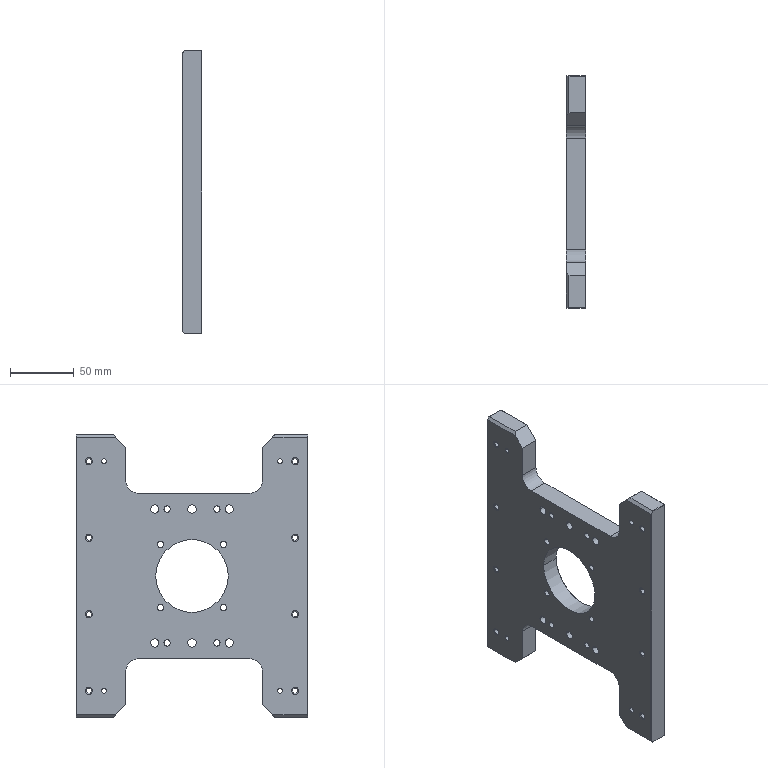Part | NX | 1 solid | 152 faces | box 15 x 182 x 222 mm | volume 407415 mm3 | cylinder 70 | cone 42 | plane 40 | commonest cylinder face diameters 4.2 x16 5 x16 6.5 x12 11 x12 4 x8 20 x4